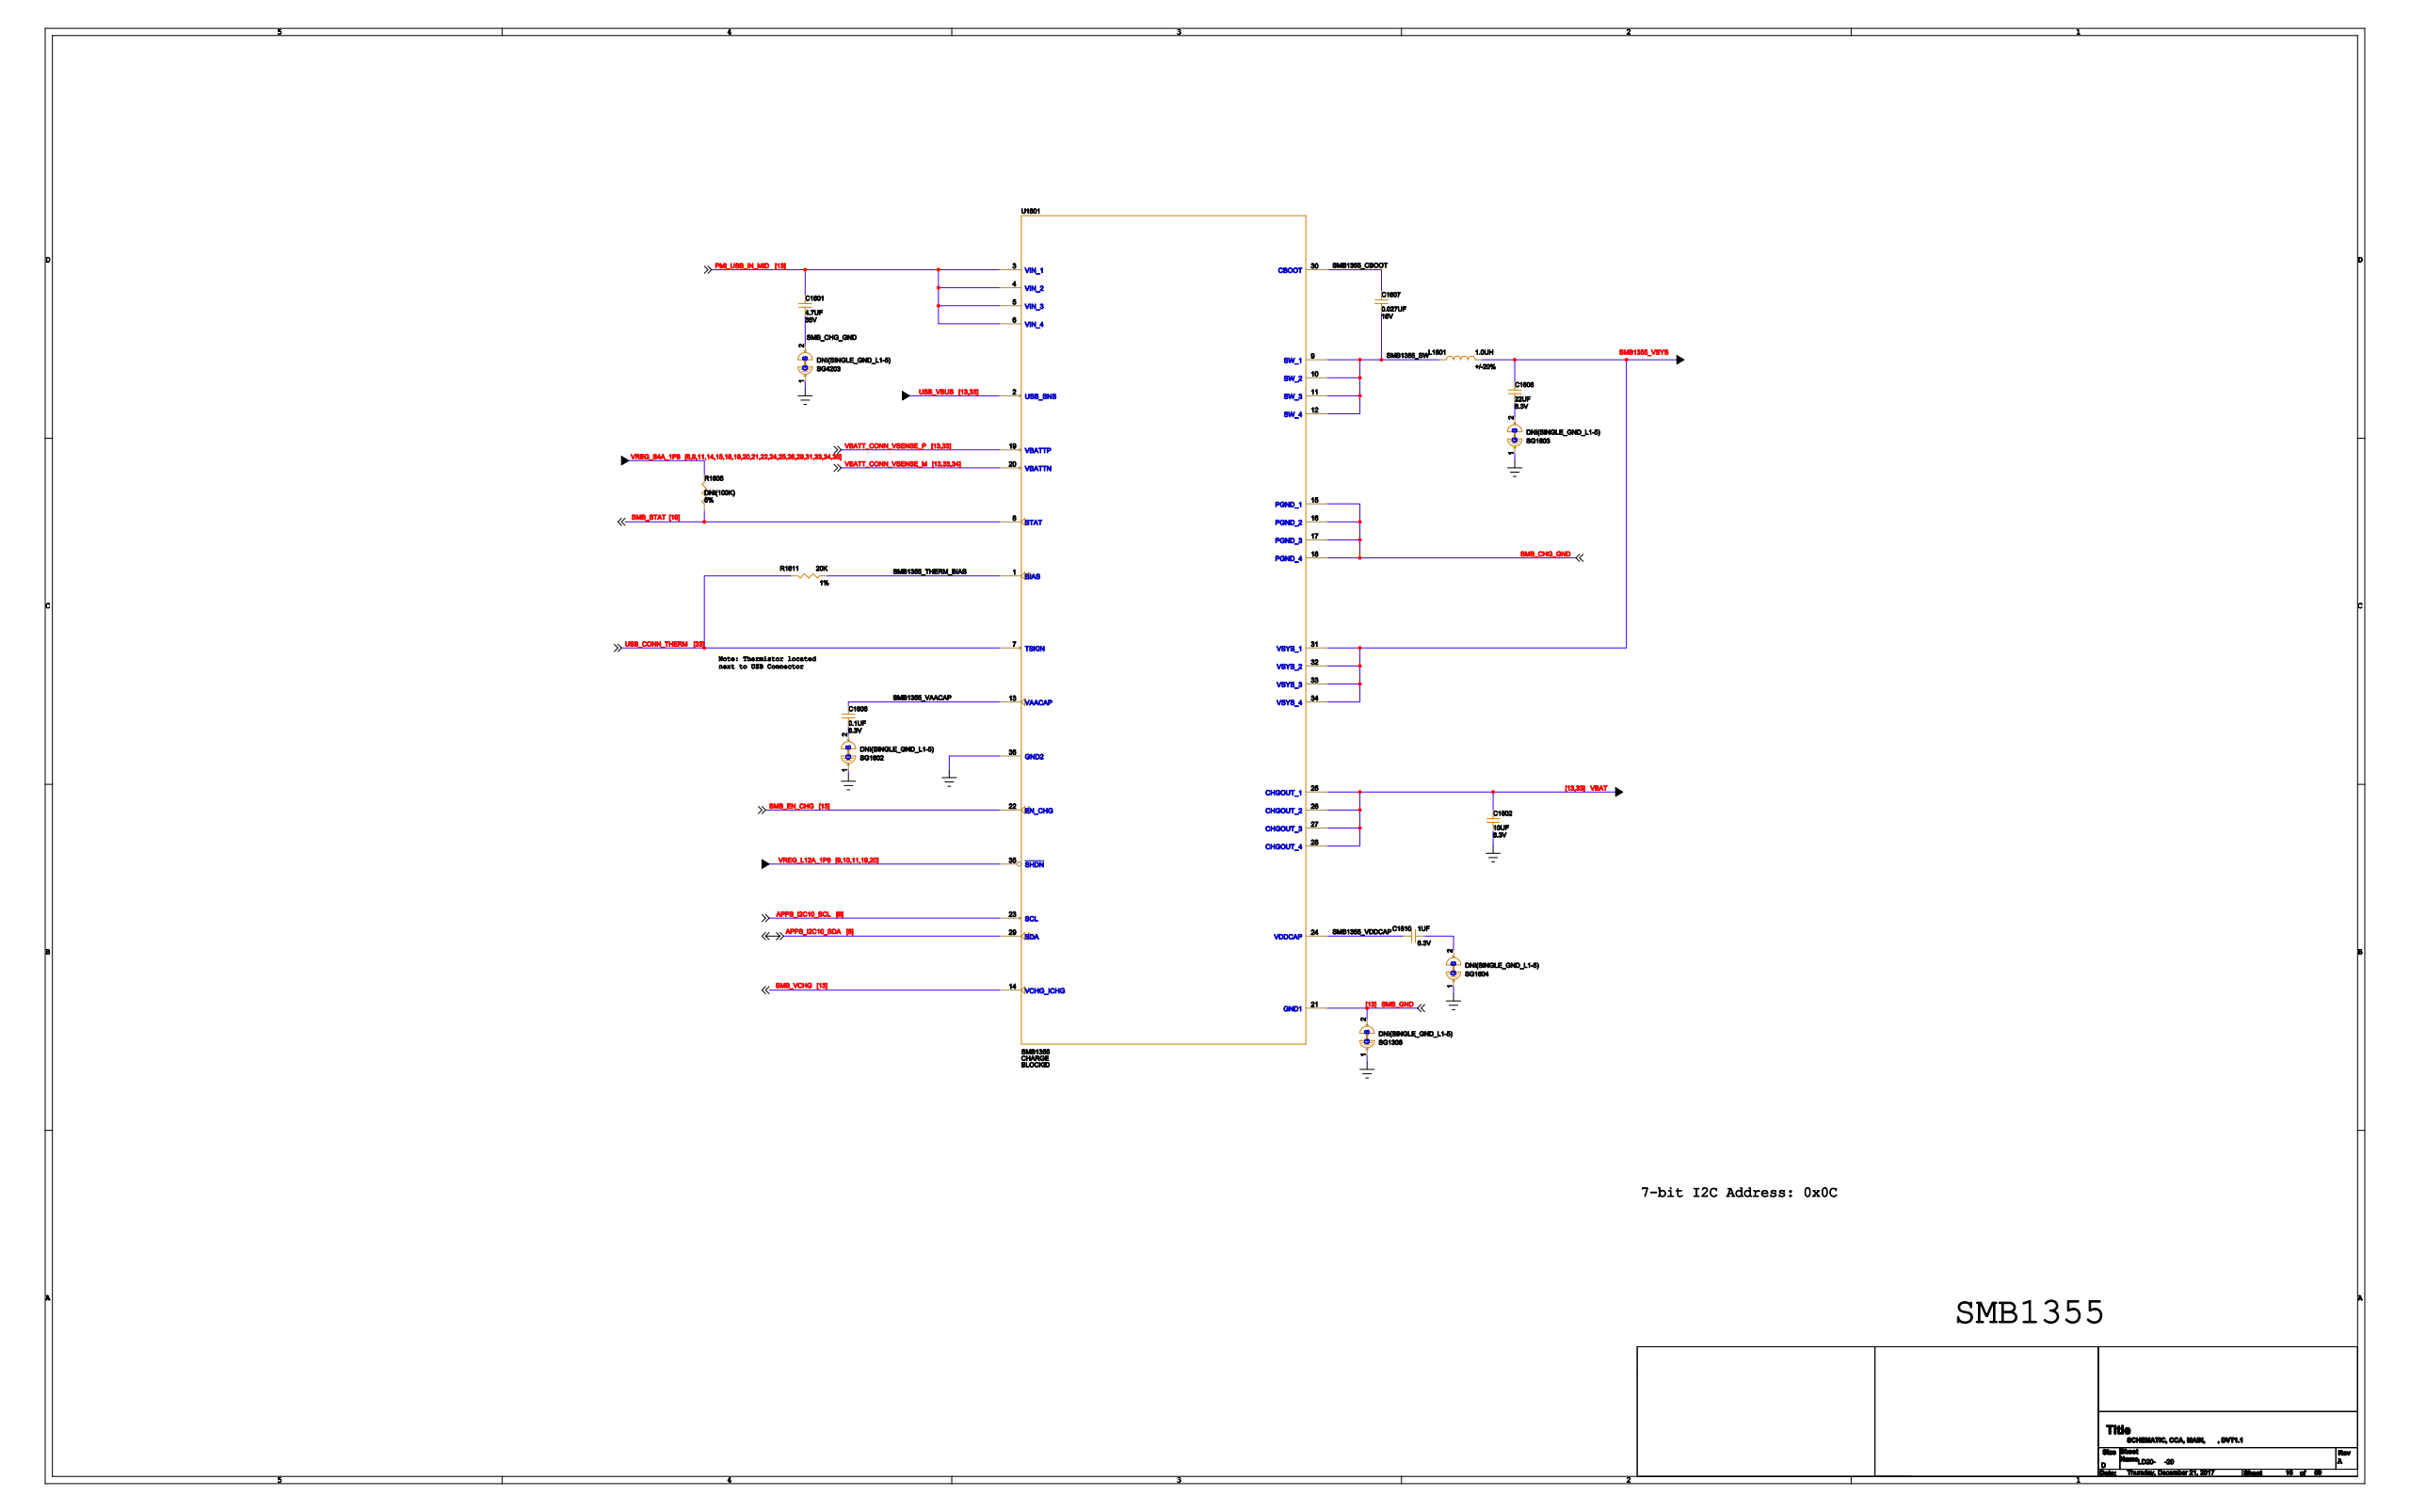Circuit board | Cadence Allegro | 1520 parts | 1149 nets | one sheet of the schematic
Parts on this sheet (reference | value | footprint):
C1601 | 4.7UF | 2P0603R
C1602 | 10UF | 2P0402RV1
C1606 | 0.1UF | 2P0201R
C1607 | 0.027UF | 2P0402R
C1608 | 22UF | 2P0603R
C1610 | 1UF | 2P0201R
L1601 | 1.0UH | 2PSM106X87RV3
R1605 | DNI(100K) | 2P0201R_DNI
R1611 | 20K | 2P0201R
SG1306 | DNI(SINGLE_GND_L1-5) | GND_L1-5
SG1602 | DNI(SINGLE_GND_L1-5) | GND_L1-5
SG1603 | DNI(SINGLE_GND_L1-5) | GND_L1-5
SG1604 | DNI(SINGLE_GND_L1-5) | GND_L1-5
SG4203 | DNI(SINGLE_GND_L1-5) | GND_L1-5
U1601 | SMB1355 | 36PGA105X105B157
Nets of these parts (net: part-pin ...):
GND: C1602-2 SG1306-1 SG1602-1 SG1603-1 SG1604-1 SG4203-1 U1601-36
VREG_S4A_1P8: R1605-1
SMB_GND: SG1306-2 U1601-21
N51215887: C1606-2 SG1602-2
N51010571: C1608-2 SG1603-2
N47040390: C1610-2 SG1604-2
SMB_CHG_GND: C1601-2 SG4203-2 U1601-15 U1601-16 U1601-17 U1601-18
VBAT: C1602-1 U1601-25 U1601-26 U1601-27 U1601-28
VBATT_CONN_VSENSE_P: U1601-19
VBATT_CONN_VSENSE_M: U1601-20
SMB1355_THERM_BIAS: R1611-2 U1601-1
SMB1355_CBOOT: C1607-1 U1601-30
SMB_EN_CHG: U1601-22
APPS_I2C10_SCL: U1601-23
APPS_I2C10_SDA: U1601-29
SMB_STAT: R1605-2 U1601-8
SMB1355_SW: C1607-2 L1601-1 U1601-9 U1601-10 U1601-11 U1601-12
VREG_L12A_1P8: U1601-35
USB_CONN_THERM: R1611-1 U1601-7
USB_VBUS: U1601-2
SMB1355_VAACAP: C1606-1 U1601-13
SMB_VCHG: U1601-14
SMB1355_VDDCAP: C1610-1 U1601-24
PMI_USB_IN_MID: C1601-1 U1601-3 U1601-4 U1601-5 U1601-6
SMB1355_VSYS: C1608-1 L1601-2 U1601-31 U1601-32 U1601-33 U1601-34